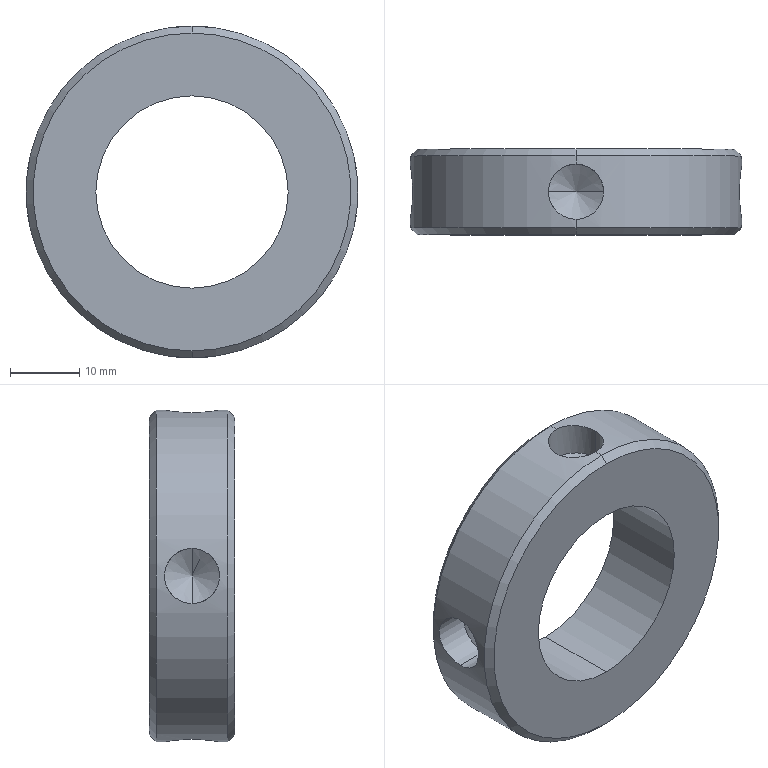Part | SolidWorks | features BaseBody 1 | 1 solid | 26 faces | box 48 x 12.4 x 48 mm | volume 13595 mm3 | cylinder 12 | cone 12 | plane 2 | commonest cylinder face diameters 8 x8 27.835 x2 48 x2
STEP:
#1=CARTESIAN_POINT('',(0.,6.2,13.918));
#2=VERTEX_POINT('',#1);
#3=CARTESIAN_POINT('',(0.,6.2,-13.918));
#4=VERTEX_POINT('',#3);
#5=CARTESIAN_POINT('',(0.,6.2,0.));
#6=DIRECTION('',(0.,-1.,0.));
#7=DIRECTION('',(0.,0.,-1.));
#8=AXIS2_PLACEMENT_3D('',#5,#6,#7);
#9=CIRCLE('',#8,13.918);
#10=EDGE_CURVE('',#2,#4,#9,.T.);
#11=ORIENTED_EDGE('',*,*,#10,.F.);
#12=CARTESIAN_POINT('',(0.,-6.2,13.918));
#13=VERTEX_POINT('',#12);
#14=CARTESIAN_POINT('',(0.,6.2,13.918));
#15=DIRECTION('',(0.,-1.,0.));
#16=VECTOR('',#15,1000.);
#17=LINE('',#14,#16);
#18=EDGE_CURVE('',#2,#13,#17,.T.);
#19=ORIENTED_EDGE('',*,*,#18,.T.);
#20=CARTESIAN_POINT('',(0.,-6.2,-13.918));
#21=VERTEX_POINT('',#20);
#22=CARTESIAN_POINT('',(0.,-6.2,0.));
#23=DIRECTION('',(0.,1.,0.));
#24=DIRECTION('',(0.,0.,-1.));
#25=AXIS2_PLACEMENT_3D('',#22,#23,#24);
#26=CIRCLE('',#25,13.918);
#27=EDGE_CURVE('',#21,#13,#26,.T.);
#28=ORIENTED_EDGE('',*,*,#27,.F.);
#29=CARTESIAN_POINT('',(0.,6.2,-13.918));
#30=DIRECTION('',(0.,-1.,0.));
#31=VECTOR('',#30,1000.);
#32=LINE('',#29,#31);
#33=EDGE_CURVE('',#4,#21,#32,.T.);
#34=ORIENTED_EDGE('',*,*,#33,.F.);
#35=EDGE_LOOP('',(#11,#19,#28,#34));
#36=FACE_OUTER_BOUND('',#35,.T.);
#37=CARTESIAN_POINT('',(0.,6.2,0.));
#38=DIRECTION('',(0.,-1.,0.));
#39=DIRECTION('',(0.,0.,-1.));
#40=AXIS2_PLACEMENT_3D('',#37,#38,#39);
#41=CYLINDRICAL_SURFACE('',#40,13.918);
#42=ADVANCED_FACE('',(#36),#41,.F.);
#43=CARTESIAN_POINT('',(0.,6.2,23.));
#44=VERTEX_POINT('',#43);
#45=CARTESIAN_POINT('',(0.,6.2,-23.));
#46=VERTEX_POINT('',#45);
#47=CARTESIAN_POINT('',(0.,6.2,0.));
#48=DIRECTION('',(0.,1.,0.));
#49=DIRECTION('',(0.,0.,-1.));
#50=AXIS2_PLACEMENT_3D('',#47,#48,#49);
#51=CIRCLE('',#50,23.);
#52=EDGE_CURVE('',#44,#46,#51,.T.);
#53=ORIENTED_EDGE('',*,*,#52,.F.);
#54=CARTESIAN_POINT('',(0.,5.2,24.));
#55=VERTEX_POINT('',#54);
#56=CARTESIAN_POINT('',(0.,5.2,24.));
#57=DIRECTION('',(0.,-0.7071,0.7071));
#58=VECTOR('',#57,1000.);
#59=LINE('',#56,#58);
#60=EDGE_CURVE('',#44,#55,#59,.T.);
#61=ORIENTED_EDGE('',*,*,#60,.T.);
#62=CARTESIAN_POINT('',(0.,5.2,-24.));
#63=VERTEX_POINT('',#62);
#64=CARTESIAN_POINT('',(0.,5.2,0.));
#65=DIRECTION('',(0.,1.,0.));
#66=DIRECTION('',(0.,0.,-1.));
#67=AXIS2_PLACEMENT_3D('',#64,#65,#66);
#68=CIRCLE('',#67,24.);
#69=EDGE_CURVE('',#55,#63,#68,.T.);
#70=ORIENTED_EDGE('',*,*,#69,.T.);
#71=CARTESIAN_POINT('',(0.,5.2,-24.));
#72=DIRECTION('',(0.,-0.7071,-0.7071));
#73=VECTOR('',#72,1000.);
#74=LINE('',#71,#73);
#75=EDGE_CURVE('',#46,#63,#74,.T.);
#76=ORIENTED_EDGE('',*,*,#75,.F.);
#77=EDGE_LOOP('',(#53,#61,#70,#76));
#78=FACE_OUTER_BOUND('',#77,.T.);
#79=CARTESIAN_POINT('',(0.,5.2,0.));
#80=DIRECTION('',(0.,-1.,0.));
#81=DIRECTION('',(0.,0.,-1.));
#82=AXIS2_PLACEMENT_3D('',#79,#80,#81);
#83=CONICAL_SURFACE('',#82,24.,0.7854);
#84=ADVANCED_FACE('',(#78),#83,.T.);
#85=CARTESIAN_POINT('',(23.664,0.,-4.));
#86=VERTEX_POINT('',#85);
#87=CARTESIAN_POINT('',(23.664,0.,4.));
#88=VERTEX_POINT('',#87);
#89=CARTESIAN_POINT('',(23.664,0.,-4.));
#90=CARTESIAN_POINT('',(23.664,-0.2647,-4.));
#91=CARTESIAN_POINT('',(23.669,-0.5249,-3.974));
#92=CARTESIAN_POINT('',(23.686,-1.037,-3.872));
#93=CARTESIAN_POINT('',(23.698,-1.291,-3.795));
#94=CARTESIAN_POINT('',(23.73,-1.775,-3.594));
#95=CARTESIAN_POINT('',(23.748,-2.005,-3.471));
#96=CARTESIAN_POINT('',(23.789,-2.439,-3.181));
#97=CARTESIAN_POINT('',(23.811,-2.644,-3.013));
#98=CARTESIAN_POINT('',(23.855,-3.013,-2.644));
#99=CARTESIAN_POINT('',(23.876,-3.178,-2.443));
#100=CARTESIAN_POINT('',(23.917,-3.47,-2.006));
#101=CARTESIAN_POINT('',(23.936,-3.594,-1.774));
#102=CARTESIAN_POINT('',(23.966,-3.794,-1.293));
#103=CARTESIAN_POINT('',(23.979,-3.871,-1.041));
#104=CARTESIAN_POINT('',(23.996,-3.974,-0.5242));
#105=CARTESIAN_POINT('',(24.,-4.,-0.2644));
#106=CARTESIAN_POINT('',(24.,-4.,0.2583));
#107=CARTESIAN_POINT('',(23.996,-3.974,0.5238));
#108=CARTESIAN_POINT('',(23.979,-3.872,1.037));
#109=CARTESIAN_POINT('',(23.967,-3.796,1.287));
#110=CARTESIAN_POINT('',(23.936,-3.596,1.771));
#111=CARTESIAN_POINT('',(23.917,-3.471,2.005));
#112=CARTESIAN_POINT('',(23.877,-3.182,2.438));
#113=CARTESIAN_POINT('',(23.855,-3.016,2.64));
#114=CARTESIAN_POINT('',(23.811,-2.644,3.013));
#115=CARTESIAN_POINT('',(23.789,-2.443,3.178));
#116=CARTESIAN_POINT('',(23.749,-2.01,3.468));
#117=CARTESIAN_POINT('',(23.73,-1.776,3.594));
#118=CARTESIAN_POINT('',(23.698,-1.292,3.795));
#119=CARTESIAN_POINT('',(23.686,-1.043,3.87));
#120=CARTESIAN_POINT('',(23.669,-0.5297,3.973));
#121=CARTESIAN_POINT('',(23.664,-0.2647,4.));
#122=CARTESIAN_POINT('',(23.664,0.,4.));
#123=B_SPLINE_CURVE_WITH_KNOTS('',3,(#89,#90,#91,#92,#93,#94,#95,#96,#97,#98,#99,#100,#101,#102,#103,#104,#105,#106,#107,#108,#109,#110,#111,#112,#113,#114,#115,#116,#117,#118,#119,#120,#121,#122),.UNSPECIFIED.,.F.,.F.,(4,2,2,2,2,2,2,2,2,2,2,2,2,2,2,2,4),(0.01252,0.01331,0.01409,0.01487,0.01566,0.01644,0.01722,0.018,0.01879,0.01957,0.02035,0.02114,0.02192,0.0227,0.02348,0.02427,0.02505),.UNSPECIFIED.);
#124=EDGE_CURVE('',#86,#88,#123,.T.);
#125=ORIENTED_EDGE('',*,*,#124,.T.);
#126=CARTESIAN_POINT('',(23.664,0.,4.));
#127=CARTESIAN_POINT('',(23.664,0.2647,4.));
#128=CARTESIAN_POINT('',(23.669,0.5249,3.974));
#129=CARTESIAN_POINT('',(23.686,1.037,3.872));
#130=CARTESIAN_POINT('',(23.698,1.291,3.795));
#131=CARTESIAN_POINT('',(23.73,1.775,3.594));
#132=CARTESIAN_POINT('',(23.748,2.005,3.471));
#133=CARTESIAN_POINT('',(23.789,2.439,3.181));
#134=CARTESIAN_POINT('',(23.811,2.644,3.013));
#135=CARTESIAN_POINT('',(23.855,3.013,2.644));
#136=CARTESIAN_POINT('',(23.876,3.178,2.443));
#137=CARTESIAN_POINT('',(23.917,3.47,2.006));
#138=CARTESIAN_POINT('',(23.936,3.594,1.774));
#139=CARTESIAN_POINT('',(23.966,3.794,1.293));
#140=CARTESIAN_POINT('',(23.979,3.871,1.041));
#141=CARTESIAN_POINT('',(23.996,3.974,0.5242));
#142=CARTESIAN_POINT('',(24.,4.,0.2644));
#143=CARTESIAN_POINT('',(24.,4.,-0.2583));
#144=CARTESIAN_POINT('',(23.996,3.974,-0.5238));
#145=CARTESIAN_POINT('',(23.979,3.872,-1.037));
#146=CARTESIAN_POINT('',(23.967,3.796,-1.287));
#147=CARTESIAN_POINT('',(23.936,3.596,-1.771));
#148=CARTESIAN_POINT('',(23.917,3.471,-2.005));
#149=CARTESIAN_POINT('',(23.877,3.182,-2.438));
#150=CARTESIAN_POINT('',(23.855,3.016,-2.64));
#151=CARTESIAN_POINT('',(23.811,2.644,-3.013));
#152=CARTESIAN_POINT('',(23.789,2.443,-3.178));
#153=CARTESIAN_POINT('',(23.749,2.01,-3.468));
#154=CARTESIAN_POINT('',(23.73,1.776,-3.594));
#155=CARTESIAN_POINT('',(23.698,1.292,-3.795));
#156=CARTESIAN_POINT('',(23.686,1.043,-3.87));
#157=CARTESIAN_POINT('',(23.669,0.5297,-3.973));
#158=CARTESIAN_POINT('',(23.664,0.2647,-4.));
#159=CARTESIAN_POINT('',(23.664,0.,-4.));
#160=B_SPLINE_CURVE_WITH_KNOTS('',3,(#126,#127,#128,#129,#130,#131,#132,#133,#134,#135,#136,#137,#138,#139,#140,#141,#142,#143,#144,#145,#146,#147,#148,#149,#150,#151,#152,#153,#154,#155,#156,#157,#158,#159),.UNSPECIFIED.,.F.,.F.,(4,2,2,2,2,2,2,2,2,2,2,2,2,2,2,2,4),(0.,0.0007828,0.001566,0.002348,0.003131,0.003914,0.004697,0.005479,0.006262,0.007045,0.007828,0.008611,0.009393,0.01018,0.01096,0.01174,0.01252),.UNSPECIFIED.);
#161=EDGE_CURVE('',#88,#86,#160,.T.);
#162=ORIENTED_EDGE('',*,*,#161,.T.);
#163=EDGE_LOOP('',(#125,#162));
#164=FACE_BOUND('',#163,.T.);
#165=ORIENTED_EDGE('',*,*,#69,.F.);
#166=CARTESIAN_POINT('',(0.,4.,24.));
#167=VERTEX_POINT('',#166);
#168=CARTESIAN_POINT('',(0.,6.2,24.));
#169=DIRECTION('',(0.,-1.,0.));
#170=VECTOR('',#169,1000.);
#171=LINE('',#168,#170);
#172=EDGE_CURVE('',#55,#167,#171,.T.);
#173=ORIENTED_EDGE('',*,*,#172,.T.);
#174=CARTESIAN_POINT('',(4.,0.,23.664));
#175=VERTEX_POINT('',#174);
#176=CARTESIAN_POINT('',(0.,4.,24.));
#177=CARTESIAN_POINT('',(0.2646,4.,24.));
#178=CARTESIAN_POINT('',(0.5247,3.974,23.996));
#179=CARTESIAN_POINT('',(1.036,3.872,23.979));
#180=CARTESIAN_POINT('',(1.29,3.795,23.967));
#181=CARTESIAN_POINT('',(1.774,3.594,23.936));
#182=CARTESIAN_POINT('',(2.004,3.472,23.917));
#183=CARTESIAN_POINT('',(2.438,3.182,23.877));
#184=CARTESIAN_POINT('',(2.643,3.013,23.855));
#185=CARTESIAN_POINT('',(3.012,2.645,23.811));
#186=CARTESIAN_POINT('',(3.177,2.444,23.789));
#187=CARTESIAN_POINT('',(3.47,2.008,23.748));
#188=CARTESIAN_POINT('',(3.594,1.776,23.73));
#189=CARTESIAN_POINT('',(3.793,1.295,23.699));
#190=CARTESIAN_POINT('',(3.871,1.043,23.686));
#191=CARTESIAN_POINT('',(3.974,0.5262,23.669));
#192=CARTESIAN_POINT('',(4.,0.2646,23.664));
#193=CARTESIAN_POINT('',(4.,0.,23.664));
#194=B_SPLINE_CURVE_WITH_KNOTS('',3,(#176,#177,#178,#179,#180,#181,#182,#183,#184,#185,#186,#187,#188,#189,#190,#191,#192,#193),.UNSPECIFIED.,.F.,.F.,(4,2,2,2,2,2,2,2,4),(-0.006259,-0.005477,-0.004695,-0.003912,-0.00313,-0.002347,-0.001565,-0.0007824,0.),.UNSPECIFIED.);
#195=EDGE_CURVE('',#167,#175,#194,.T.);
#196=ORIENTED_EDGE('',*,*,#195,.T.);
#197=CARTESIAN_POINT('',(0.,-4.,24.));
#198=VERTEX_POINT('',#197);
#199=CARTESIAN_POINT('',(4.,0.,23.664));
#200=CARTESIAN_POINT('',(4.,-0.2646,23.664));
#201=CARTESIAN_POINT('',(3.974,-0.5247,23.669));
#202=CARTESIAN_POINT('',(3.872,-1.036,23.686));
#203=CARTESIAN_POINT('',(3.795,-1.29,23.698));
#204=CARTESIAN_POINT('',(3.594,-1.774,23.73));
#205=CARTESIAN_POINT('',(3.472,-2.004,23.748));
#206=CARTESIAN_POINT('',(3.182,-2.438,23.789));
#207=CARTESIAN_POINT('',(3.013,-2.643,23.811));
#208=CARTESIAN_POINT('',(2.645,-3.012,23.854));
#209=CARTESIAN_POINT('',(2.444,-3.177,23.876));
#210=CARTESIAN_POINT('',(2.008,-3.47,23.917));
#211=CARTESIAN_POINT('',(1.776,-3.594,23.935));
#212=CARTESIAN_POINT('',(1.295,-3.793,23.966));
#213=CARTESIAN_POINT('',(1.043,-3.871,23.979));
#214=CARTESIAN_POINT('',(0.5262,-3.974,23.996));
#215=CARTESIAN_POINT('',(0.2646,-4.,24.));
#216=CARTESIAN_POINT('',(0.,-4.,24.));
#217=B_SPLINE_CURVE_WITH_KNOTS('',3,(#199,#200,#201,#202,#203,#204,#205,#206,#207,#208,#209,#210,#211,#212,#213,#214,#215,#216),.UNSPECIFIED.,.F.,.F.,(4,2,2,2,2,2,2,2,4),(0.,0.0007824,0.001565,0.002347,0.00313,0.003912,0.004695,0.005477,0.00626),.UNSPECIFIED.);
#218=EDGE_CURVE('',#175,#198,#217,.T.);
#219=ORIENTED_EDGE('',*,*,#218,.T.);
#220=CARTESIAN_POINT('',(0.,-5.2,24.));
#221=VERTEX_POINT('',#220);
#222=CARTESIAN_POINT('',(0.,6.2,24.));
#223=DIRECTION('',(0.,-1.,0.));
#224=VECTOR('',#223,1000.);
#225=LINE('',#222,#224);
#226=EDGE_CURVE('',#198,#221,#225,.T.);
#227=ORIENTED_EDGE('',*,*,#226,.T.);
#228=CARTESIAN_POINT('',(0.,-5.2,-24.));
#229=VERTEX_POINT('',#228);
#230=CARTESIAN_POINT('',(0.,-5.2,0.));
#231=DIRECTION('',(0.,1.,0.));
#232=DIRECTION('',(0.,0.,-1.));
#233=AXIS2_PLACEMENT_3D('',#230,#231,#232);
#234=CIRCLE('',#233,24.);
#235=EDGE_CURVE('',#221,#229,#234,.T.);
#236=ORIENTED_EDGE('',*,*,#235,.T.);
#237=CARTESIAN_POINT('',(0.,-4.,-24.));
#238=VERTEX_POINT('',#237);
#239=CARTESIAN_POINT('',(0.,6.2,-24.));
#240=DIRECTION('',(0.,-1.,0.));
#241=VECTOR('',#240,1000.);
#242=LINE('',#239,#241);
#243=EDGE_CURVE('',#238,#229,#242,.T.);
#244=ORIENTED_EDGE('',*,*,#243,.F.);
#245=CARTESIAN_POINT('',(4.,0.,-23.664));
#246=VERTEX_POINT('',#245);
#247=CARTESIAN_POINT('',(0.,-4.,-24.));
#248=CARTESIAN_POINT('',(0.2646,-4.,-24.));
#249=CARTESIAN_POINT('',(0.5247,-3.974,-23.996));
#250=CARTESIAN_POINT('',(1.036,-3.872,-23.979));
#251=CARTESIAN_POINT('',(1.29,-3.795,-23.967));
#252=CARTESIAN_POINT('',(1.774,-3.594,-23.936));
#253=CARTESIAN_POINT('',(2.004,-3.472,-23.917));
#254=CARTESIAN_POINT('',(2.438,-3.182,-23.877));
#255=CARTESIAN_POINT('',(2.643,-3.013,-23.855));
#256=CARTESIAN_POINT('',(3.012,-2.645,-23.811));
#257=CARTESIAN_POINT('',(3.177,-2.444,-23.789));
#258=CARTESIAN_POINT('',(3.47,-2.008,-23.748));
#259=CARTESIAN_POINT('',(3.594,-1.776,-23.73));
#260=CARTESIAN_POINT('',(3.793,-1.295,-23.699));
#261=CARTESIAN_POINT('',(3.871,-1.043,-23.686));
#262=CARTESIAN_POINT('',(3.974,-0.5262,-23.669));
#263=CARTESIAN_POINT('',(4.,-0.2646,-23.664));
#264=CARTESIAN_POINT('',(4.,0.,-23.664));
#265=B_SPLINE_CURVE_WITH_KNOTS('',3,(#247,#248,#249,#250,#251,#252,#253,#254,#255,#256,#257,#258,#259,#260,#261,#262,#263,#264),.UNSPECIFIED.,.F.,.F.,(4,2,2,2,2,2,2,2,4),(-0.006259,-0.005477,-0.004695,-0.003912,-0.00313,-0.002347,-0.001565,-0.0007824,0.),.UNSPECIFIED.);
#266=EDGE_CURVE('',#238,#246,#265,.T.);
#267=ORIENTED_EDGE('',*,*,#266,.T.);
#268=CARTESIAN_POINT('',(0.,4.,-24.));
#269=VERTEX_POINT('',#268);
#270=CARTESIAN_POINT('',(4.,0.,-23.664));
#271=CARTESIAN_POINT('',(4.,0.2646,-23.664));
#272=CARTESIAN_POINT('',(3.974,0.5247,-23.669));
#273=CARTESIAN_POINT('',(3.872,1.036,-23.686));
#274=CARTESIAN_POINT('',(3.795,1.29,-23.698));
#275=CARTESIAN_POINT('',(3.594,1.774,-23.73));
#276=CARTESIAN_POINT('',(3.472,2.004,-23.748));
#277=CARTESIAN_POINT('',(3.182,2.438,-23.789));
#278=CARTESIAN_POINT('',(3.013,2.643,-23.811));
#279=CARTESIAN_POINT('',(2.645,3.012,-23.854));
#280=CARTESIAN_POINT('',(2.444,3.177,-23.876));
#281=CARTESIAN_POINT('',(2.008,3.47,-23.917));
#282=CARTESIAN_POINT('',(1.776,3.594,-23.935));
#283=CARTESIAN_POINT('',(1.295,3.793,-23.966));
#284=CARTESIAN_POINT('',(1.043,3.871,-23.979));
#285=CARTESIAN_POINT('',(0.5262,3.974,-23.996));
#286=CARTESIAN_POINT('',(0.2646,4.,-24.));
#287=CARTESIAN_POINT('',(0.,4.,-24.));
#288=B_SPLINE_CURVE_WITH_KNOTS('',3,(#270,#271,#272,#273,#274,#275,#276,#277,#278,#279,#280,#281,#282,#283,#284,#285,#286,#287),.UNSPECIFIED.,.F.,.F.,(4,2,2,2,2,2,2,2,4),(0.,0.0007824,0.001565,0.002347,0.00313,0.003912,0.004695,0.005477,0.00626),.UNSPECIFIED.);
#289=EDGE_CURVE('',#246,#269,#288,.T.);
#290=ORIENTED_EDGE('',*,*,#289,.T.);
#291=CARTESIAN_POINT('',(0.,6.2,-24.));
#292=DIRECTION('',(0.,-1.,0.));
#293=VECTOR('',#292,1000.);
#294=LINE('',#291,#293);
#295=EDGE_CURVE('',#63,#269,#294,.T.);
#296=ORIENTED_EDGE('',*,*,#295,.F.);
#297=EDGE_LOOP('',(#165,#173,#196,#219,#227,#236,#244,#267,#290,#296));
#298=FACE_OUTER_BOUND('',#297,.T.);
#299=CARTESIAN_POINT('',(0.,6.2,0.));
#300=DIRECTION('',(0.,-1.,0.));
#301=DIRECTION('',(0.,0.,-1.));
#302=AXIS2_PLACEMENT_3D('',#299,#300,#301);
#303=CYLINDRICAL_SURFACE('',#302,24.);
#304=ADVANCED_FACE('',(#164,#298),#303,.T.);
#305=CARTESIAN_POINT('',(0.,-6.2,23.));
#306=VERTEX_POINT('',#305);
#307=CARTESIAN_POINT('',(0.,-6.2,-23.));
#308=VERTEX_POINT('',#307);
#309=CARTESIAN_POINT('',(0.,-6.2,0.));
#310=DIRECTION('',(0.,1.,0.));
#311=DIRECTION('',(0.,0.,1.));
#312=AXIS2_PLACEMENT_3D('',#309,#310,#311);
#313=CIRCLE('',#312,23.);
#314=EDGE_CURVE('',#306,#308,#313,.T.);
#315=ORIENTED_EDGE('',*,*,#314,.T.);
#316=CARTESIAN_POINT('',(0.,-5.2,-24.));
#317=DIRECTION('',(0.,0.7071,-0.7071));
#318=VECTOR('',#317,1000.);
#319=LINE('',#316,#318);
#320=EDGE_CURVE('',#308,#229,#319,.T.);
#321=ORIENTED_EDGE('',*,*,#320,.T.);
#322=ORIENTED_EDGE('',*,*,#235,.F.);
#323=CARTESIAN_POINT('',(0.,-5.2,24.));
#324=DIRECTION('',(0.,0.7071,0.7071));
#325=VECTOR('',#324,1000.);
#326=LINE('',#323,#325);
#327=EDGE_CURVE('',#306,#221,#326,.T.);
#328=ORIENTED_EDGE('',*,*,#327,.F.);
#329=EDGE_LOOP('',(#315,#321,#322,#328));
#330=FACE_OUTER_BOUND('',#329,.T.);
#331=CARTESIAN_POINT('',(0.,-5.2,0.));
#332=DIRECTION('',(0.,1.,0.));
#333=DIRECTION('',(0.,0.,1.));
#334=AXIS2_PLACEMENT_3D('',#331,#332,#333);
#335=CONICAL_SURFACE('',#334,24.,0.7854);
#336=ADVANCED_FACE('',(#330),#335,.T.);
#337=CARTESIAN_POINT('',(4.,0.,-19.));
#338=VERTEX_POINT('',#337);
#339=CARTESIAN_POINT('',(-4.,0.,-19.));
#340=VERTEX_POINT('',#339);
#341=CARTESIAN_POINT('',(0.,0.,-19.));
#342=DIRECTION('',(0.,0.,-1.));
#343=DIRECTION('',(-1.,0.,0.));
#344=AXIS2_PLACEMENT_3D('',#341,#342,#343);
#345=CIRCLE('',#344,4.);
#346=EDGE_CURVE('',#338,#340,#345,.T.);
#347=ORIENTED_EDGE('',*,*,#346,.F.);
#348=CARTESIAN_POINT('',(4.,0.,-24.));
#349=DIRECTION('',(0.,0.,-1.));
#350=VECTOR('',#349,1000.);
#351=LINE('',#348,#350);
#352=EDGE_CURVE('',#338,#246,#351,.T.);
#353=ORIENTED_EDGE('',*,*,#352,.T.);
#354=ORIENTED_EDGE('',*,*,#266,.F.);
#355=CARTESIAN_POINT('',(-4.,0.,-23.664));
#356=VERTEX_POINT('',#355);
#357=CARTESIAN_POINT('',(-4.,0.,-23.664));
#358=CARTESIAN_POINT('',(-4.,-0.2646,-23.664));
#359=CARTESIAN_POINT('',(-3.974,-0.5247,-23.669));
#360=CARTESIAN_POINT('',(-3.872,-1.036,-23.686));
#361=CARTESIAN_POINT('',(-3.795,-1.29,-23.698));
#362=CARTESIAN_POINT('',(-3.594,-1.774,-23.73));
#363=CARTESIAN_POINT('',(-3.472,-2.004,-23.748));
#364=CARTESIAN_POINT('',(-3.182,-2.438,-23.789));
#365=CARTESIAN_POINT('',(-3.013,-2.643,-23.811));
#366=CARTESIAN_POINT('',(-2.645,-3.012,-23.854));
#367=CARTESIAN_POINT('',(-2.444,-3.177,-23.876));
#368=CARTESIAN_POINT('',(-2.008,-3.47,-23.917));
#369=CARTESIAN_POINT('',(-1.776,-3.594,-23.935));
#370=CARTESIAN_POINT('',(-1.295,-3.793,-23.966));
#371=CARTESIAN_POINT('',(-1.043,-3.871,-23.979));
#372=CARTESIAN_POINT('',(-0.5262,-3.974,-23.996));
#373=CARTESIAN_POINT('',(-0.2646,-4.,-24.));
#374=CARTESIAN_POINT('',(0.,-4.,-24.));
#375=B_SPLINE_CURVE_WITH_KNOTS('',3,(#357,#358,#359,#360,#361,#362,#363,#364,#365,#366,#367,#368,#369,#370,#371,#372,#373,#374),.UNSPECIFIED.,.F.,.F.,(4,2,2,2,2,2,2,2,4),(0.01252,0.0133,0.01408,0.01487,0.01565,0.01643,0.01721,0.018,0.01878),.UNSPECIFIED.);
#376=EDGE_CURVE('',#356,#238,#375,.T.);
#377=ORIENTED_EDGE('',*,*,#376,.F.);
#378=CARTESIAN_POINT('',(-4.,0.,-24.));
#379=DIRECTION('',(0.,0.,-1.));
#380=VECTOR('',#379,1000.);
#381=LINE('',#378,#380);
#382=EDGE_CURVE('',#340,#356,#381,.T.);
#383=ORIENTED_EDGE('',*,*,#382,.F.);
#384=EDGE_LOOP('',(#347,#353,#354,#377,#383));
#385=FACE_OUTER_BOUND('',#384,.T.);
#386=CARTESIAN_POINT('',(0.,0.,-24.));
#387=DIRECTION('',(0.,0.,-1.));
#388=DIRECTION('',(-1.,0.,0.));
#389=AXIS2_PLACEMENT_3D('',#386,#387,#388);
#390=CYLINDRICAL_SURFACE('',#389,4.);
#391=ADVANCED_FACE('',(#385),#390,.F.);
#392=CARTESIAN_POINT('',(-4.,0.,19.));
#393=VERTEX_POINT('',#392);
#394=CARTESIAN_POINT('',(4.,0.,19.));
#395=VERTEX_POINT('',#394);
#396=CARTESIAN_POINT('',(0.,0.,19.));
#397=DIRECTION('',(0.,0.,1.));
#398=DIRECTION('',(1.,0.,0.));
#399=AXIS2_PLACEMENT_3D('',#396,#397,#398);
#400=CIRCLE('',#399,4.);
#401=EDGE_CURVE('',#393,#395,#400,.T.);
#402=ORIENTED_EDGE('',*,*,#401,.F.);
#403=CARTESIAN_POINT('',(-4.,0.,23.664));
#404=VERTEX_POINT('',#403);
#405=CARTESIAN_POINT('',(-4.,0.,24.));
#406=DIRECTION('',(0.,0.,1.));
#407=VECTOR('',#406,1000.);
#408=LINE('',#405,#407);
#409=EDGE_CURVE('',#393,#404,#408,.T.);
#410=ORIENTED_EDGE('',*,*,#409,.T.);
#411=CARTESIAN_POINT('',(0.,-4.,24.));
#412=CARTESIAN_POINT('',(-0.2646,-4.,24.));
#413=CARTESIAN_POINT('',(-0.5247,-3.974,23.996));
#414=CARTESIAN_POINT('',(-1.036,-3.872,23.979));
#415=CARTESIAN_POINT('',(-1.29,-3.795,23.967));
#416=CARTESIAN_POINT('',(-1.774,-3.594,23.936));
#417=CARTESIAN_POINT('',(-2.004,-3.472,23.917));
#418=CARTESIAN_POINT('',(-2.438,-3.182,23.877));
#419=CARTESIAN_POINT('',(-2.643,-3.013,23.855));
#420=CARTESIAN_POINT('',(-3.012,-2.645,23.811));
#421=CARTESIAN_POINT('',(-3.177,-2.444,23.789));
#422=CARTESIAN_POINT('',(-3.47,-2.008,23.748));
#423=CARTESIAN_POINT('',(-3.594,-1.776,23.73));
#424=CARTESIAN_POINT('',(-3.793,-1.295,23.699));
#425=CARTESIAN_POINT('',(-3.871,-1.043,23.686));
#426=CARTESIAN_POINT('',(-3.974,-0.5262,23.669));
#427=CARTESIAN_POINT('',(-4.,-0.2646,23.664));
#428=CARTESIAN_POINT('',(-4.,0.,23.664));
#429=B_SPLINE_CURVE_WITH_KNOTS('',3,(#411,#412,#413,#414,#415,#416,#417,#418,#419,#420,#421,#422,#423,#424,#425,#426,#427,#428),.UNSPECIFIED.,.F.,.F.,(4,2,2,2,2,2,2,2,4),(0.00626,0.007042,0.007824,0.008607,0.009389,0.01017,0.01095,0.01174,0.01252),.UNSPECIFIED.);
#430=EDGE_CURVE('',#198,#404,#429,.T.);
#431=ORIENTED_EDGE('',*,*,#430,.F.);
#432=ORIENTED_EDGE('',*,*,#218,.F.);
#433=CARTESIAN_POINT('',(4.,0.,24.));
#434=DIRECTION('',(0.,0.,1.));
#435=VECTOR('',#434,1000.);
#436=LINE('',#433,#435);
#437=EDGE_CURVE('',#395,#175,#436,.T.);
#438=ORIENTED_EDGE('',*,*,#437,.F.);
#439=EDGE_LOOP('',(#402,#410,#431,#432,#438));
#440=FACE_OUTER_BOUND('',#439,.T.);
#441=CARTESIAN_POINT('',(0.,0.,24.));
#442=DIRECTION('',(0.,0.,1.));
#443=DIRECTION('',(1.,0.,0.));
#444=AXIS2_PLACEMENT_3D('',#441,#442,#443);
#445=CYLINDRICAL_SURFACE('',#444,4.);
#446=ADVANCED_FACE('',(#440),#445,.F.);
#447=CARTESIAN_POINT('',(19.,0.,4.));
#448=VERTEX_POINT('',#447);
#449=CARTESIAN_POINT('',(19.,0.,-4.));
#450=VERTEX_POINT('',#449);
#451=CARTESIAN_POINT('',(19.,0.,0.));
#452=DIRECTION('',(1.,0.,0.));
#453=DIRECTION('',(0.,0.,-1.));
#454=AXIS2_PLACEMENT_3D('',#451,#452,#453);
#455=CIRCLE('',#454,4.);
#456=EDGE_CURVE('',#448,#450,#455,.T.);
#457=ORIENTED_EDGE('',*,*,#456,.F.);
#458=CARTESIAN_POINT('',(24.,0.,4.));
#459=DIRECTION('',(1.,0.,0.));
#460=VECTOR('',#459,1000.);
#461=LINE('',#458,#460);
#462=EDGE_CURVE('',#448,#88,#461,.T.);
#463=ORIENTED_EDGE('',*,*,#462,.T.);
#464=ORIENTED_EDGE('',*,*,#124,.F.);
#465=CARTESIAN_POINT('',(24.,0.,-4.));
#466=DIRECTION('',(1.,0.,0.));
#467=VECTOR('',#466,1000.);
#468=LINE('',#465,#467);
#469=EDGE_CURVE('',#450,#86,#468,.T.);
#470=ORIENTED_EDGE('',*,*,#469,.F.);
#471=EDGE_LOOP('',(#457,#463,#464,#470));
#472=FACE_OUTER_BOUND('',#471,.T.);
#473=CARTESIAN_POINT('',(24.,0.,0.));
#474=DIRECTION('',(1.,0.,0.));
#475=DIRECTION('',(0.,0.,-1.));
#476=AXIS2_PLACEMENT_3D('',#473,#474,#475);
#477=CYLINDRICAL_SURFACE('',#476,4.);
#478=ADVANCED_FACE('',(#472),#477,.F.);
#479=CARTESIAN_POINT('',(-19.,0.,-4.));
#480=VERTEX_POINT('',#479);
#481=CARTESIAN_POINT('',(-19.,0.,4.));
#482=VERTEX_POINT('',#481);
#483=CARTESIAN_POINT('',(-19.,0.,0.));
#484=DIRECTION('',(-1.,0.,0.));
#485=DIRECTION('',(0.,0.,1.));
#486=AXIS2_PLACEMENT_3D('',#483,#484,#485);
#487=CIRCLE('',#486,4.);
#488=EDGE_CURVE('',#480,#482,#487,.T.);
#489=ORIENTED_EDGE('',*,*,#488,.F.);
#490=CARTESIAN_POINT('',(-23.664,0.,-4.));
#491=VERTEX_POINT('',#490);
#492=CARTESIAN_POINT('',(-24.,0.,-4.));
#493=DIRECTION('',(-1.,0.,0.));
#494=VECTOR('',#493,1000.);
#495=LINE('',#492,#494);
#496=EDGE_CURVE('',#480,#491,#495,.T.);
#497=ORIENTED_EDGE('',*,*,#496,.T.);
#498=CARTESIAN_POINT('',(-23.664,0.,4.));
#499=VERTEX_POINT('',#498);
#500=CARTESIAN_POINT('',(-23.664,0.,4.));
#501=CARTESIAN_POINT('',(-23.664,-0.2647,4.));
#502=CARTESIAN_POINT('',(-23.669,-0.5249,3.974));
#503=CARTESIAN_POINT('',(-23.686,-1.037,3.872));
#504=CARTESIAN_POINT('',(-23.698,-1.291,3.795));
#505=CARTESIAN_POINT('',(-23.73,-1.775,3.594));
#506=CARTESIAN_POINT('',(-23.748,-2.005,3.471));
#507=CARTESIAN_POINT('',(-23.789,-2.439,3.181));
#508=CARTESIAN_POINT('',(-23.811,-2.644,3.013));
#509=CARTESIAN_POINT('',(-23.855,-3.013,2.644));
#510=CARTESIAN_POINT('',(-23.876,-3.178,2.443));
#511=CARTESIAN_POINT('',(-23.917,-3.47,2.006));
#512=CARTESIAN_POINT('',(-23.936,-3.594,1.774));
#513=CARTESIAN_POINT('',(-23.966,-3.794,1.293));
#514=CARTESIAN_POINT('',(-23.979,-3.871,1.041));
#515=CARTESIAN_POINT('',(-23.996,-3.974,0.5242));
#516=CARTESIAN_POINT('',(-24.,-4.,0.2644));
#517=CARTESIAN_POINT('',(-24.,-4.,-0.2583));
#518=CARTESIAN_POINT('',(-23.996,-3.974,-0.5238));
#519=CARTESIAN_POINT('',(-23.979,-3.872,-1.037));
#520=CARTESIAN_POINT('',(-23.967,-3.796,-1.287));
#521=CARTESIAN_POINT('',(-23.936,-3.596,-1.771));
#522=CARTESIAN_POINT('',(-23.917,-3.471,-2.005));
#523=CARTESIAN_POINT('',(-23.877,-3.182,-2.438));
#524=CARTESIAN_POINT('',(-23.855,-3.016,-2.64));
#525=CARTESIAN_POINT('',(-23.811,-2.644,-3.013));
#526=CARTESIAN_POINT('',(-23.789,-2.443,-3.178));
#527=CARTESIAN_POINT('',(-23.749,-2.01,-3.468));
#528=CARTESIAN_POINT('',(-23.73,-1.776,-3.594));
#529=CARTESIAN_POINT('',(-23.698,-1.292,-3.795));
#530=CARTESIAN_POINT('',(-23.686,-1.043,-3.87));
#531=CARTESIAN_POINT('',(-23.669,-0.5297,-3.973));
#532=CARTESIAN_POINT('',(-23.664,-0.2647,-4.));
#533=CARTESIAN_POINT('',(-23.664,0.,-4.));
#534=B_SPLINE_CURVE_WITH_KNOTS('',3,(#500,#501,#502,#503,#504,#505,#506,#507,#508,#509,#510,#511,#512,#513,#514,#515,#516,#517,#518,#519,#520,#521,#522,#523,#524,#525,#526,#527,#528,#529,#530,#531,#532,#533),.UNSPECIFIED.,.F.,.F.,(4,2,2,2,2,2,2,2,2,2,2,2,2,2,2,2,4),(0.01252,0.01331,0.01409,0.01487,0.01566,0.01644,0.01722,0.018,0.01879,0.01957,0.02035,0.02114,0.02192,0.0227,0.02348,0.02427,0.02505),.UNSPECIFIED.);
#535=EDGE_CURVE('',#499,#491,#534,.T.);
#536=ORIENTED_EDGE('',*,*,#535,.F.);
#537=CARTESIAN_POINT('',(-24.,0.,4.));
#538=DIRECTION('',(-1.,0.,0.));
#539=VECTOR('',#538,1000.);
#540=LINE('',#537,#539);
#541=EDGE_CURVE('',#482,#499,#540,.T.);
#542=ORIENTED_EDGE('',*,*,#541,.F.);
#543=EDGE_LOOP('',(#489,#497,#536,#542));
#544=FACE_OUTER_BOUND('',#543,.T.);
#545=CARTESIAN_POINT('',(-24.,0.,0.));
#546=DIRECTION('',(-1.,0.,0.));
#547=DIRECTION('',(0.,0.,1.));
#548=AXIS2_PLACEMENT_3D('',#545,#546,#547);
#549=CYLINDRICAL_SURFACE('',#548,4.);
#550=ADVANCED_FACE('',(#544),#549,.F.);
#551=CARTESIAN_POINT('',(0.,0.,-16.597));
#552=VERTEX_POINT('',#551);
#553=CARTESIAN_POINT('',(-4.,0.,-19.));
#554=DIRECTION('',(-0.8572,0.,-0.515));
#555=VECTOR('',#554,1000.);
#556=LINE('',#553,#555);
#557=EDGE_CURVE('',#552,#340,#556,.T.);
#558=ORIENTED_EDGE('',*,*,#557,.F.);
#559=CARTESIAN_POINT('',(4.,0.,-19.));
#560=DIRECTION('',(0.8572,0.,-0.515));
#561=VECTOR('',#560,1000.);
#562=LINE('',#559,#561);
#563=EDGE_CURVE('',#552,#338,#562,.T.);
#564=ORIENTED_EDGE('',*,*,#563,.T.);
#565=ORIENTED_EDGE('',*,*,#346,.T.);
#566=EDGE_LOOP('',(#558,#564,#565));
#567=FACE_OUTER_BOUND('',#566,.T.);
#568=CARTESIAN_POINT('',(0.,0.,-19.));
#569=DIRECTION('',(0.,0.,-1.));
#570=DIRECTION('',(-1.,0.,0.));
#571=AXIS2_PLACEMENT_3D('',#568,#569,#570);
#572=CONICAL_SURFACE('',#571,4.,1.03);
#573=ADVANCED_FACE('',(#567),#572,.F.);
#574=CARTESIAN_POINT('',(0.,0.,16.597));
#575=VERTEX_POINT('',#574);
#576=CARTESIAN_POINT('',(4.,0.,19.));
#577=DIRECTION('',(0.8572,0.,0.515));
#578=VECTOR('',#577,1000.);
#579=LINE('',#576,#578);
#580=EDGE_CURVE('',#575,#395,#579,.T.);
#581=ORIENTED_EDGE('',*,*,#580,.F.);
#582=CARTESIAN_POINT('',(-4.,0.,19.));
#583=DIRECTION('',(-0.8572,0.,0.515));
#584=VECTOR('',#583,1000.);
#585=LINE('',#582,#584);
#586=EDGE_CURVE('',#575,#393,#585,.T.);
#587=ORIENTED_EDGE('',*,*,#586,.T.);
#588=ORIENTED_EDGE('',*,*,#401,.T.);
#589=EDGE_LOOP('',(#581,#587,#588));
#590=FACE_OUTER_BOUND('',#589,.T.);
#591=CARTESIAN_POINT('',(0.,0.,19.));
#592=DIRECTION('',(0.,0.,1.));
#593=DIRECTION('',(1.,0.,0.));
#594=AXIS2_PLACEMENT_3D('',#591,#592,#593);
#595=CONICAL_SURFACE('',#594,4.,1.03);
#596=ADVANCED_FACE('',(#590),#595,.F.);
#597=CARTESIAN_POINT('',(16.597,0.,0.));
#598=VERTEX_POINT('',#597);
#599=CARTESIAN_POINT('',(19.,0.,-4.));
#600=DIRECTION('',(0.515,0.,-0.8572));
#601=VECTOR('',#600,1000.);
#602=LINE('',#599,#601);
#603=EDGE_CURVE('',#598,#450,#602,.T.);
#604=ORIENTED_EDGE('',*,*,#603,.F.);
#605=CARTESIAN_POINT('',(19.,0.,4.));
#606=DIRECTION('',(0.515,0.,0.8572));
#607=VECTOR('',#606,1000.);
#608=LINE('',#605,#607);
#609=EDGE_CURVE('',#598,#448,#608,.T.);
#610=ORIENTED_EDGE('',*,*,#609,.T.);
#611=ORIENTED_EDGE('',*,*,#456,.T.);
#612=EDGE_LOOP('',(#604,#610,#611));
#613=FACE_OUTER_BOUND('',#612,.T.);
#614=CARTESIAN_POINT('',(19.,0.,0.));
#615=DIRECTION('',(1.,0.,0.));
#616=DIRECTION('',(0.,0.,-1.));
#617=AXIS2_PLACEMENT_3D('',#614,#615,#616);
#618=CONICAL_SURFACE('',#617,4.,1.03);
#619=ADVANCED_FACE('',(#613),#618,.F.);
#620=CARTESIAN_POINT('',(-16.597,0.,0.));
#621=VERTEX_POINT('',#620);
#622=CARTESIAN_POINT('',(-19.,0.,4.));
#623=DIRECTION('',(-0.515,0.,0.8572));
#624=VECTOR('',#623,1000.);
#625=LINE('',#622,#624);
#626=EDGE_CURVE('',#621,#482,#625,.T.);
#627=ORIENTED_EDGE('',*,*,#626,.F.);
#628=CARTESIAN_POINT('',(-19.,0.,-4.));
#629=DIRECTION('',(-0.515,0.,-0.8572));
#630=VECTOR('',#629,1000.);
#631=LINE('',#628,#630);
#632=EDGE_CURVE('',#621,#480,#631,.T.);
#633=ORIENTED_EDGE('',*,*,#632,.T.);
#634=ORIENTED_EDGE('',*,*,#488,.T.);
#635=EDGE_LOOP('',(#627,#633,#634));
#636=FACE_OUTER_BOUND('',#635,.T.);
#637=CARTESIAN_POINT('',(-19.,0.,0.));
#638=DIRECTION('',(-1.,0.,0.));
#639=DIRECTION('',(0.,0.,1.));
#640=AXIS2_PLACEMENT_3D('',#637,#638,#639);
#641=CONICAL_SURFACE('',#640,4.,1.03);
#642=ADVANCED_FACE('',(#636),#641,.F.);
#643=CARTESIAN_POINT('',(0.,6.2,0.));
#644=DIRECTION('',(0.,-1.,0.));
#645=DIRECTION('',(0.,0.,-1.));
#646=AXIS2_PLACEMENT_3D('',#643,#644,#645);
#647=CIRCLE('',#646,13.918);
#648=EDGE_CURVE('',#4,#2,#647,.T.);
#649=ORIENTED_EDGE('',*,*,#648,.T.);
#650=ORIENTED_EDGE('',*,*,#10,.T.);
#651=EDGE_LOOP('',(#649,#650));
#652=FACE_BOUND('',#651,.T.);
#653=CARTESIAN_POINT('',(0.,6.2,0.));
#654=DIRECTION('',(0.,1.,0.));
#655=DIRECTION('',(0.,0.,-1.));
#656=AXIS2_PLACEMENT_3D('',#653,#654,#655);
#657=CIRCLE('',#656,23.);
#658=EDGE_CURVE('',#46,#44,#657,.T.);
#659=ORIENTED_EDGE('',*,*,#658,.T.);
#660=ORIENTED_EDGE('',*,*,#52,.T.);
#661=EDGE_LOOP('',(#659,#660));
#662=FACE_OUTER_BOUND('',#661,.T.);
#663=CARTESIAN_POINT('',(0.,6.2,0.));
#664=DIRECTION('',(0.,1.,0.));
#665=DIRECTION('',(0.,0.,1.));
#666=AXIS2_PLACEMENT_3D('',#663,#664,#665);
#667=PLANE('',#666);
#668=ADVANCED_FACE('',(#652,#662),#667,.T.);
#669=ORIENTED_EDGE('',*,*,#18,.F.);
#670=ORIENTED_EDGE('',*,*,#648,.F.);
#671=ORIENTED_EDGE('',*,*,#33,.T.);
#672=CARTESIAN_POINT('',(0.,-6.2,0.));
#673=DIRECTION('',(0.,1.,0.));
#674=DIRECTION('',(0.,0.,-1.));
#675=AXIS2_PLACEMENT_3D('',#672,#673,#674);
#676=CIRCLE('',#675,13.918);
#677=EDGE_CURVE('',#13,#21,#676,.T.);
#678=ORIENTED_EDGE('',*,*,#677,.F.);
#679=EDGE_LOOP('',(#669,#670,#671,#678));
#680=FACE_OUTER_BOUND('',#679,.T.);
#681=CARTESIAN_POINT('',(0.,6.2,0.));
#682=DIRECTION('',(0.,-1.,0.));
#683=DIRECTION('',(0.,0.,-1.));
#684=AXIS2_PLACEMENT_3D('',#681,#682,#683);
#685=CYLINDRICAL_SURFACE('',#684,13.918);
#686=ADVANCED_FACE('',(#680),#685,.F.);
#687=ORIENTED_EDGE('',*,*,#60,.F.);
#688=ORIENTED_EDGE('',*,*,#658,.F.);
#689=ORIENTED_EDGE('',*,*,#75,.T.);
#690=CARTESIAN_POINT('',(0.,5.2,0.));
#691=DIRECTION('',(0.,1.,0.));
#692=DIRECTION('',(0.,0.,-1.));
#693=AXIS2_PLACEMENT_3D('',#690,#691,#692);
#694=CIRCLE('',#693,24.);
#695=EDGE_CURVE('',#63,#55,#694,.T.);
#696=ORIENTED_EDGE('',*,*,#695,.T.);
#697=EDGE_LOOP('',(#687,#688,#689,#696));
#698=FACE_OUTER_BOUND('',#697,.T.);
#699=CARTESIAN_POINT('',(0.,5.2,0.));
#700=DIRECTION('',(0.,-1.,0.));
#701=DIRECTION('',(0.,0.,-1.));
#702=AXIS2_PLACEMENT_3D('',#699,#700,#701);
#703=CONICAL_SURFACE('',#702,24.,0.7854);
#704=ADVANCED_FACE('',(#698),#703,.T.);
#705=ORIENTED_EDGE('',*,*,#27,.T.);
#706=ORIENTED_EDGE('',*,*,#677,.T.);
#707=EDGE_LOOP('',(#705,#706));
#708=FACE_BOUND('',#707,.T.);
#709=ORIENTED_EDGE('',*,*,#314,.F.);
#710=CARTESIAN_POINT('',(0.,-6.2,0.));
#711=DIRECTION('',(0.,1.,0.));
#712=DIRECTION('',(0.,0.,1.));
#713=AXIS2_PLACEMENT_3D('',#710,#711,#712);
#714=CIRCLE('',#713,23.);
#715=EDGE_CURVE('',#308,#306,#714,.T.);
#716=ORIENTED_EDGE('',*,*,#715,.F.);
#717=EDGE_LOOP('',(#709,#716));
#718=FACE_OUTER_BOUND('',#717,.T.);
#719=CARTESIAN_POINT('',(0.,-6.2,0.));
#720=DIRECTION('',(0.,1.,0.));
#721=DIRECTION('',(0.,0.,1.));
#722=AXIS2_PLACEMENT_3D('',#719,#720,#721);
#723=PLANE('',#722);
#724=ADVANCED_FACE('',(#708,#718),#723,.F.);
#725=ORIENTED_EDGE('',*,*,#172,.F.);
#726=ORIENTED_EDGE('',*,*,#695,.F.);
#727=ORIENTED_EDGE('',*,*,#295,.T.);
#728=CARTESIAN_POINT('',(0.,4.,-24.));
#729=CARTESIAN_POINT('',(-0.2646,4.,-24.));
#730=CARTESIAN_POINT('',(-0.5247,3.974,-23.996));
#731=CARTESIAN_POINT('',(-1.036,3.872,-23.979));
#732=CARTESIAN_POINT('',(-1.29,3.795,-23.967));
#733=CARTESIAN_POINT('',(-1.774,3.594,-23.936));
#734=CARTESIAN_POINT('',(-2.004,3.472,-23.917));
#735=CARTESIAN_POINT('',(-2.438,3.182,-23.877));
#736=CARTESIAN_POINT('',(-2.643,3.013,-23.855));
#737=CARTESIAN_POINT('',(-3.012,2.645,-23.811));
#738=CARTESIAN_POINT('',(-3.177,2.444,-23.789));
#739=CARTESIAN_POINT('',(-3.47,2.008,-23.748));
#740=CARTESIAN_POINT('',(-3.594,1.776,-23.73));
#741=CARTESIAN_POINT('',(-3.793,1.295,-23.699));
#742=CARTESIAN_POINT('',(-3.871,1.043,-23.686));
#743=CARTESIAN_POINT('',(-3.974,0.5262,-23.669));
#744=CARTESIAN_POINT('',(-4.,0.2646,-23.664));
#745=CARTESIAN_POINT('',(-4.,0.,-23.664));
#746=B_SPLINE_CURVE_WITH_KNOTS('',3,(#728,#729,#730,#731,#732,#733,#734,#735,#736,#737,#738,#739,#740,#741,#742,#743,#744,#745),.UNSPECIFIED.,.F.,.F.,(4,2,2,2,2,2,2,2,4),(0.00626,0.007042,0.007824,0.008607,0.009389,0.01017,0.01095,0.01174,0.01252),.UNSPECIFIED.);
#747=EDGE_CURVE('',#269,#356,#746,.T.);
#748=ORIENTED_EDGE('',*,*,#747,.T.);
#749=ORIENTED_EDGE('',*,*,#376,.T.);
#750=ORIENTED_EDGE('',*,*,#243,.T.);
#751=CARTESIAN_POINT('',(0.,-5.2,0.));
#752=DIRECTION('',(0.,1.,0.));
#753=DIRECTION('',(0.,0.,-1.));
#754=AXIS2_PLACEMENT_3D('',#751,#752,#753);
#755=CIRCLE('',#754,24.);
#756=EDGE_CURVE('',#229,#221,#755,.T.);
#757=ORIENTED_EDGE('',*,*,#756,.T.);
#758=ORIENTED_EDGE('',*,*,#226,.F.);
#759=ORIENTED_EDGE('',*,*,#430,.T.);
#760=CARTESIAN_POINT('',(-4.,0.,23.664));
#761=CARTESIAN_POINT('',(-4.,0.2646,23.664));
#762=CARTESIAN_POINT('',(-3.974,0.5247,23.669));
#763=CARTESIAN_POINT('',(-3.872,1.036,23.686));
#764=CARTESIAN_POINT('',(-3.795,1.29,23.698));
#765=CARTESIAN_POINT('',(-3.594,1.774,23.73));
#766=CARTESIAN_POINT('',(-3.472,2.004,23.748));
#767=CARTESIAN_POINT('',(-3.182,2.438,23.789));
#768=CARTESIAN_POINT('',(-3.013,2.643,23.811));
#769=CARTESIAN_POINT('',(-2.645,3.012,23.854));
#770=CARTESIAN_POINT('',(-2.444,3.177,23.876));
#771=CARTESIAN_POINT('',(-2.008,3.47,23.917));
#772=CARTESIAN_POINT('',(-1.776,3.594,23.935));
#773=CARTESIAN_POINT('',(-1.295,3.793,23.966));
#774=CARTESIAN_POINT('',(-1.043,3.871,23.979));
#775=CARTESIAN_POINT('',(-0.5262,3.974,23.996));
#776=CARTESIAN_POINT('',(-0.2646,4.,24.));
#777=CARTESIAN_POINT('',(0.,4.,24.));
#778=B_SPLINE_CURVE_WITH_KNOTS('',3,(#760,#761,#762,#763,#764,#765,#766,#767,#768,#769,#770,#771,#772,#773,#774,#775,#776,#777),.UNSPECIFIED.,.F.,.F.,(4,2,2,2,2,2,2,2,4),(0.01252,0.0133,0.01408,0.01487,0.01565,0.01643,0.01721,0.018,0.01878),.UNSPECIFIED.);
#779=EDGE_CURVE('',#404,#167,#778,.T.);
#780=ORIENTED_EDGE('',*,*,#779,.T.);
#781=EDGE_LOOP('',(#725,#726,#727,#748,#749,#750,#757,#758,#759,#780));
#782=FACE_OUTER_BOUND('',#781,.T.);
#783=ORIENTED_EDGE('',*,*,#535,.T.);
#784=CARTESIAN_POINT('',(-23.664,0.,-4.));
#785=CARTESIAN_POINT('',(-23.664,0.2647,-4.));
#786=CARTESIAN_POINT('',(-23.669,0.5249,-3.974));
#787=CARTESIAN_POINT('',(-23.686,1.037,-3.872));
#788=CARTESIAN_POINT('',(-23.698,1.291,-3.795));
#789=CARTESIAN_POINT('',(-23.73,1.775,-3.594));
#790=CARTESIAN_POINT('',(-23.748,2.005,-3.471));
#791=CARTESIAN_POINT('',(-23.789,2.439,-3.181));
#792=CARTESIAN_POINT('',(-23.811,2.644,-3.013));
#793=CARTESIAN_POINT('',(-23.855,3.013,-2.644));
#794=CARTESIAN_POINT('',(-23.876,3.178,-2.443));
#795=CARTESIAN_POINT('',(-23.917,3.47,-2.006));
#796=CARTESIAN_POINT('',(-23.936,3.594,-1.774));
#797=CARTESIAN_POINT('',(-23.966,3.794,-1.293));
#798=CARTESIAN_POINT('',(-23.979,3.871,-1.041));
#799=CARTESIAN_POINT('',(-23.996,3.974,-0.5242));
#800=CARTESIAN_POINT('',(-24.,4.,-0.2644));
#801=CARTESIAN_POINT('',(-24.,4.,0.2583));
#802=CARTESIAN_POINT('',(-23.996,3.974,0.5238));
#803=CARTESIAN_POINT('',(-23.979,3.872,1.037));
#804=CARTESIAN_POINT('',(-23.967,3.796,1.287));
#805=CARTESIAN_POINT('',(-23.936,3.596,1.771));
#806=CARTESIAN_POINT('',(-23.917,3.471,2.005));
#807=CARTESIAN_POINT('',(-23.877,3.182,2.438));
#808=CARTESIAN_POINT('',(-23.855,3.016,2.64));
#809=CARTESIAN_POINT('',(-23.811,2.644,3.013));
#810=CARTESIAN_POINT('',(-23.789,2.443,3.178));
#811=CARTESIAN_POINT('',(-23.749,2.01,3.468));
#812=CARTESIAN_POINT('',(-23.73,1.776,3.594));
#813=CARTESIAN_POINT('',(-23.698,1.292,3.795));
#814=CARTESIAN_POINT('',(-23.686,1.043,3.87));
#815=CARTESIAN_POINT('',(-23.669,0.5297,3.973));
#816=CARTESIAN_POINT('',(-23.664,0.2647,4.));
#817=CARTESIAN_POINT('',(-23.664,0.,4.));
#818=B_SPLINE_CURVE_WITH_KNOTS('',3,(#784,#785,#786,#787,#788,#789,#790,#791,#792,#793,#794,#795,#796,#797,#798,#799,#800,#801,#802,#803,#804,#805,#806,#807,#808,#809,#810,#811,#812,#813,#814,#815,#816,#817),.UNSPECIFIED.,.F.,.F.,(4,2,2,2,2,2,2,2,2,2,2,2,2,2,2,2,4),(0.,0.0007828,0.001566,0.002348,0.003131,0.003914,0.004697,0.005479,0.006262,0.007045,0.007828,0.008611,0.009393,0.01018,0.01096,0.01174,0.01252),.UNSPECIFIED.);
#819=EDGE_CURVE('',#491,#499,#818,.T.);
#820=ORIENTED_EDGE('',*,*,#819,.T.);
#821=EDGE_LOOP('',(#783,#820));
#822=FACE_BOUND('',#821,.T.);
#823=CARTESIAN_POINT('',(0.,6.2,0.));
#824=DIRECTION('',(0.,-1.,0.));
#825=DIRECTION('',(0.,0.,-1.));
#826=AXIS2_PLACEMENT_3D('',#823,#824,#825);
#827=CYLINDRICAL_SURFACE('',#826,24.);
#828=ADVANCED_FACE('',(#782,#822),#827,.T.);
#829=ORIENTED_EDGE('',*,*,#320,.F.);
#830=ORIENTED_EDGE('',*,*,#715,.T.);
#831=ORIENTED_EDGE('',*,*,#327,.T.);
#832=ORIENTED_EDGE('',*,*,#756,.F.);
#833=EDGE_LOOP('',(#829,#830,#831,#832));
#834=FACE_OUTER_BOUND('',#833,.T.);
#835=CARTESIAN_POINT('',(0.,-5.2,0.));
#836=DIRECTION('',(0.,1.,0.));
#837=DIRECTION('',(0.,0.,1.));
#838=AXIS2_PLACEMENT_3D('',#835,#836,#837);
#839=CONICAL_SURFACE('',#838,24.,0.7854);
#840=ADVANCED_FACE('',(#834),#839,.T.);
#841=ORIENTED_EDGE('',*,*,#352,.F.);
#842=CARTESIAN_POINT('',(0.,0.,-19.));
#843=DIRECTION('',(0.,0.,-1.));
#844=DIRECTION('',(-1.,0.,0.));
#845=AXIS2_PLACEMENT_3D('',#842,#843,#844);
#846=CIRCLE('',#845,4.);
#847=EDGE_CURVE('',#340,#338,#846,.T.);
#848=ORIENTED_EDGE('',*,*,#847,.F.);
#849=ORIENTED_EDGE('',*,*,#382,.T.);
#850=ORIENTED_EDGE('',*,*,#747,.F.);
#851=ORIENTED_EDGE('',*,*,#289,.F.);
#852=EDGE_LOOP('',(#841,#848,#849,#850,#851));
#853=FACE_OUTER_BOUND('',#852,.T.);
#854=CARTESIAN_POINT('',(0.,0.,-24.));
#855=DIRECTION('',(0.,0.,-1.));
#856=DIRECTION('',(-1.,0.,0.));
#857=AXIS2_PLACEMENT_3D('',#854,#855,#856);
#858=CYLINDRICAL_SURFACE('',#857,4.);
#859=ADVANCED_FACE('',(#853),#858,.F.);
#860=ORIENTED_EDGE('',*,*,#409,.F.);
#861=CARTESIAN_POINT('',(0.,0.,19.));
#862=DIRECTION('',(0.,0.,1.));
#863=DIRECTION('',(1.,0.,0.));
#864=AXIS2_PLACEMENT_3D('',#861,#862,#863);
#865=CIRCLE('',#864,4.);
#866=EDGE_CURVE('',#395,#393,#865,.T.);
#867=ORIENTED_EDGE('',*,*,#866,.F.);
#868=ORIENTED_EDGE('',*,*,#437,.T.);
#869=ORIENTED_EDGE('',*,*,#195,.F.);
#870=ORIENTED_EDGE('',*,*,#779,.F.);
#871=EDGE_LOOP('',(#860,#867,#868,#869,#870));
#872=FACE_OUTER_BOUND('',#871,.T.);
#873=CARTESIAN_POINT('',(0.,0.,24.));
#874=DIRECTION('',(0.,0.,1.));
#875=DIRECTION('',(1.,0.,0.));
#876=AXIS2_PLACEMENT_3D('',#873,#874,#875);
#877=CYLINDRICAL_SURFACE('',#876,4.);
#878=ADVANCED_FACE('',(#872),#877,.F.);
#879=ORIENTED_EDGE('',*,*,#462,.F.);
#880=CARTESIAN_POINT('',(19.,0.,0.));
#881=DIRECTION('',(1.,0.,0.));
#882=DIRECTION('',(0.,0.,-1.));
#883=AXIS2_PLACEMENT_3D('',#880,#881,#882);
#884=CIRCLE('',#883,4.);
#885=EDGE_CURVE('',#450,#448,#884,.T.);
#886=ORIENTED_EDGE('',*,*,#885,.F.);
#887=ORIENTED_EDGE('',*,*,#469,.T.);
#888=ORIENTED_EDGE('',*,*,#161,.F.);
#889=EDGE_LOOP('',(#879,#886,#887,#888));
#890=FACE_OUTER_BOUND('',#889,.T.);
#891=CARTESIAN_POINT('',(24.,0.,0.));
#892=DIRECTION('',(1.,0.,0.));
#893=DIRECTION('',(0.,0.,-1.));
#894=AXIS2_PLACEMENT_3D('',#891,#892,#893);
#895=CYLINDRICAL_SURFACE('',#894,4.);
#896=ADVANCED_FACE('',(#890),#895,.F.);
#897=ORIENTED_EDGE('',*,*,#496,.F.);
#898=CARTESIAN_POINT('',(-19.,0.,0.));
#899=DIRECTION('',(-1.,0.,0.));
#900=DIRECTION('',(0.,0.,1.));
#901=AXIS2_PLACEMENT_3D('',#898,#899,#900);
#902=CIRCLE('',#901,4.);
#903=EDGE_CURVE('',#482,#480,#902,.T.);
#904=ORIENTED_EDGE('',*,*,#903,.F.);
#905=ORIENTED_EDGE('',*,*,#541,.T.);
#906=ORIENTED_EDGE('',*,*,#819,.F.);
#907=EDGE_LOOP('',(#897,#904,#905,#906));
#908=FACE_OUTER_BOUND('',#907,.T.);
#909=CARTESIAN_POINT('',(-24.,0.,0.));
#910=DIRECTION('',(-1.,0.,0.));
#911=DIRECTION('',(0.,0.,1.));
#912=AXIS2_PLACEMENT_3D('',#909,#910,#911);
#913=CYLINDRICAL_SURFACE('',#912,4.);
#914=ADVANCED_FACE('',(#908),#913,.F.);
#915=ORIENTED_EDGE('',*,*,#563,.F.);
#916=ORIENTED_EDGE('',*,*,#557,.T.);
#917=ORIENTED_EDGE('',*,*,#847,.T.);
#918=EDGE_LOOP('',(#915,#916,#917));
#919=FACE_OUTER_BOUND('',#918,.T.);
#920=CARTESIAN_POINT('',(0.,0.,-19.));
#921=DIRECTION('',(0.,0.,-1.));
#922=DIRECTION('',(-1.,0.,0.));
#923=AXIS2_PLACEMENT_3D('',#920,#921,#922);
#924=CONICAL_SURFACE('',#923,4.,1.03);
#925=ADVANCED_FACE('',(#919),#924,.F.);
#926=ORIENTED_EDGE('',*,*,#586,.F.);
#927=ORIENTED_EDGE('',*,*,#580,.T.);
#928=ORIENTED_EDGE('',*,*,#866,.T.);
#929=EDGE_LOOP('',(#926,#927,#928));
#930=FACE_OUTER_BOUND('',#929,.T.);
#931=CARTESIAN_POINT('',(0.,0.,19.));
#932=DIRECTION('',(0.,0.,1.));
#933=DIRECTION('',(1.,0.,0.));
#934=AXIS2_PLACEMENT_3D('',#931,#932,#933);
#935=CONICAL_SURFACE('',#934,4.,1.03);
#936=ADVANCED_FACE('',(#930),#935,.F.);
#937=ORIENTED_EDGE('',*,*,#609,.F.);
#938=ORIENTED_EDGE('',*,*,#603,.T.);
#939=ORIENTED_EDGE('',*,*,#885,.T.);
#940=EDGE_LOOP('',(#937,#938,#939));
#941=FACE_OUTER_BOUND('',#940,.T.);
#942=CARTESIAN_POINT('',(19.,0.,0.));
#943=DIRECTION('',(1.,0.,0.));
#944=DIRECTION('',(0.,0.,-1.));
#945=AXIS2_PLACEMENT_3D('',#942,#943,#944);
#946=CONICAL_SURFACE('',#945,4.,1.03);
#947=ADVANCED_FACE('',(#941),#946,.F.);
#948=ORIENTED_EDGE('',*,*,#632,.F.);
#949=ORIENTED_EDGE('',*,*,#626,.T.);
#950=ORIENTED_EDGE('',*,*,#903,.T.);
#951=EDGE_LOOP('',(#948,#949,#950));
#952=FACE_OUTER_BOUND('',#951,.T.);
#953=CARTESIAN_POINT('',(-19.,0.,0.));
#954=DIRECTION('',(-1.,0.,0.));
#955=DIRECTION('',(0.,0.,1.));
#956=AXIS2_PLACEMENT_3D('',#953,#954,#955);
#957=CONICAL_SURFACE('',#956,4.,1.03);
#958=ADVANCED_FACE('',(#952),#957,.F.);
#959=CLOSED_SHELL('',(#42,#84,#304,#336,#391,#446,#478,#550,#573,#596,#619,#642,#668,#686,#704,#724,#828,#840,#859,#878,#896,#914,#925,#936,#947,#958));
#960=MANIFOLD_SOLID_BREP('',#959);
#961=CARTESIAN_POINT('',(0.,0.,0.));
#962=DIRECTION('',(0.,0.,1.));
#963=DIRECTION('',(1.,0.,0.));
#964=AXIS2_PLACEMENT_3D('',#961,#962,#963);
#965=(LENGTH_UNIT()NAMED_UNIT(*)SI_UNIT(.MILLI.,.METRE.));
#966=UNCERTAINTY_MEASURE_WITH_UNIT(LENGTH_MEASURE(0.00001),#965,'','');
#967=(NAMED_UNIT(*)PLANE_ANGLE_UNIT()SI_UNIT($,.RADIAN.));
#968=(NAMED_UNIT(*)SI_UNIT($,.STERADIAN.)SOLID_ANGLE_UNIT());
#969=(GEOMETRIC_REPRESENTATION_CONTEXT(3)GLOBAL_UNCERTAINTY_ASSIGNED_CONTEXT((#966))GLOBAL_UNIT_ASSIGNED_CONTEXT((#965,#967,#968))REPRESENTATION_CONTEXT('',''));
#970=ADVANCED_BREP_SHAPE_REPRESENTATION('',(#960,#964),#969);